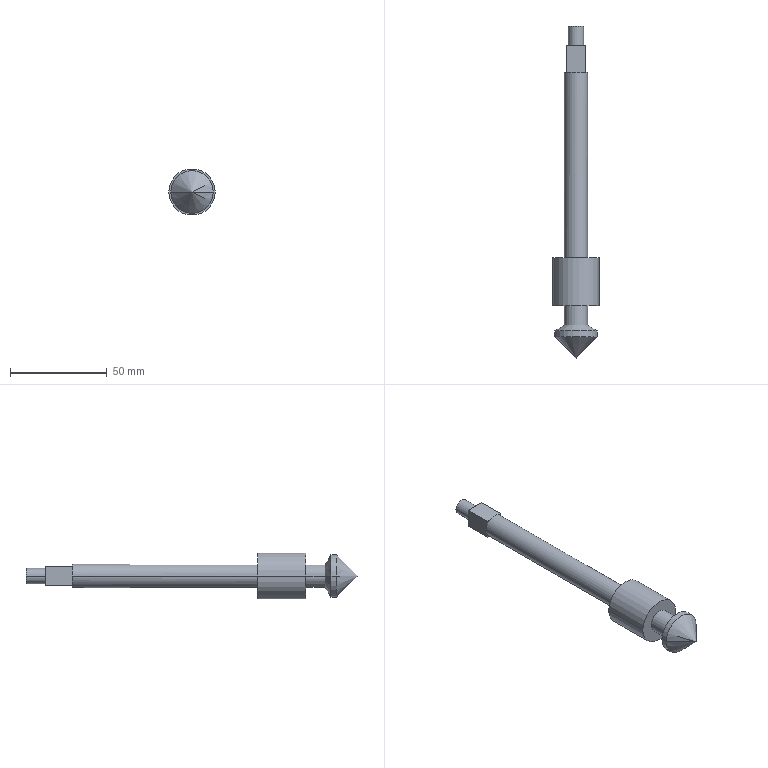Part | SolidWorks | features ICE 2, Revolution 1 | 1 solid | 30 faces | box 24 x 172 x 24 mm | volume 28435 mm3 | plane 16 | cylinder 10 | cone 4 | commonest cylinder face diameters 12 x4 8 x2 22 x2 24 x2
STEP:
#1=CARTESIAN_POINT('',(-4.,172.,0.));
#2=VERTEX_POINT('',#1);
#3=CARTESIAN_POINT('',(4.,172.,0.));
#4=VERTEX_POINT('',#3);
#5=CARTESIAN_POINT('',(0.,172.,0.));
#6=DIRECTION('',(0.,1.,0.));
#7=DIRECTION('',(-1.,0.,0.));
#8=AXIS2_PLACEMENT_3D('',#5,#6,#7);
#9=CIRCLE('',#8,4.);
#10=EDGE_CURVE('',#2,#4,#9,.T.);
#11=ORIENTED_EDGE('',*,*,#10,.F.);
#12=CARTESIAN_POINT('',(-4.,162.,0.));
#13=VERTEX_POINT('',#12);
#14=CARTESIAN_POINT('',(-4.,172.,0.));
#15=DIRECTION('',(0.,-1.,0.));
#16=VECTOR('',#15,1000.);
#17=LINE('',#14,#16);
#18=EDGE_CURVE('',#2,#13,#17,.T.);
#19=ORIENTED_EDGE('',*,*,#18,.T.);
#20=CARTESIAN_POINT('',(4.,162.,0.));
#21=VERTEX_POINT('',#20);
#22=CARTESIAN_POINT('',(0.,162.,0.));
#23=DIRECTION('',(0.,1.,0.));
#24=DIRECTION('',(1.,0.,0.));
#25=AXIS2_PLACEMENT_3D('',#22,#23,#24);
#26=CIRCLE('',#25,4.);
#27=EDGE_CURVE('',#13,#21,#26,.T.);
#28=ORIENTED_EDGE('',*,*,#27,.T.);
#29=CARTESIAN_POINT('',(4.,172.,0.));
#30=DIRECTION('',(0.,-1.,0.));
#31=VECTOR('',#30,1000.);
#32=LINE('',#29,#31);
#33=EDGE_CURVE('',#4,#21,#32,.T.);
#34=ORIENTED_EDGE('',*,*,#33,.F.);
#35=EDGE_LOOP('',(#11,#19,#28,#34));
#36=FACE_OUTER_BOUND('',#35,.T.);
#37=CARTESIAN_POINT('',(0.,172.,0.));
#38=DIRECTION('',(0.,-1.,0.));
#39=DIRECTION('',(1.,0.,0.));
#40=AXIS2_PLACEMENT_3D('',#37,#38,#39);
#41=CYLINDRICAL_SURFACE('',#40,4.);
#42=ADVANCED_FACE('',(#36),#41,.T.);
#43=CARTESIAN_POINT('',(-5.,148.,3.317));
#44=VERTEX_POINT('',#43);
#45=CARTESIAN_POINT('',(-6.,148.,0.));
#46=VERTEX_POINT('',#45);
#47=CARTESIAN_POINT('',(0.,148.,0.));
#48=DIRECTION('',(0.,-1.,0.));
#49=DIRECTION('',(1.,0.,0.));
#50=AXIS2_PLACEMENT_3D('',#47,#48,#49);
#51=CIRCLE('',#50,6.);
#52=EDGE_CURVE('',#44,#46,#51,.T.);
#53=ORIENTED_EDGE('',*,*,#52,.T.);
#54=CARTESIAN_POINT('',(-6.,52.,0.));
#55=VERTEX_POINT('',#54);
#56=CARTESIAN_POINT('',(-6.,-1000.,0.));
#57=DIRECTION('',(0.,-1.,0.));
#58=VECTOR('',#57,1000.);
#59=LINE('',#56,#58);
#60=EDGE_CURVE('',#46,#55,#59,.T.);
#61=ORIENTED_EDGE('',*,*,#60,.T.);
#62=CARTESIAN_POINT('',(6.,52.,0.));
#63=VERTEX_POINT('',#62);
#64=CARTESIAN_POINT('',(0.,52.,0.));
#65=DIRECTION('',(0.,-1.,0.));
#66=DIRECTION('',(1.,0.,0.));
#67=AXIS2_PLACEMENT_3D('',#64,#65,#66);
#68=CIRCLE('',#67,6.);
#69=EDGE_CURVE('',#63,#55,#68,.T.);
#70=ORIENTED_EDGE('',*,*,#69,.F.);
#71=CARTESIAN_POINT('',(6.,148.,0.));
#72=VERTEX_POINT('',#71);
#73=CARTESIAN_POINT('',(6.,-1000.,0.));
#74=DIRECTION('',(0.,-1.,0.));
#75=VECTOR('',#74,1000.);
#76=LINE('',#73,#75);
#77=EDGE_CURVE('',#72,#63,#76,.T.);
#78=ORIENTED_EDGE('',*,*,#77,.F.);
#79=CARTESIAN_POINT('',(5.,148.,3.317));
#80=VERTEX_POINT('',#79);
#81=CARTESIAN_POINT('',(0.,148.,0.));
#82=DIRECTION('',(0.,-1.,0.));
#83=DIRECTION('',(1.,0.,0.));
#84=AXIS2_PLACEMENT_3D('',#81,#82,#83);
#85=CIRCLE('',#84,6.);
#86=EDGE_CURVE('',#72,#80,#85,.T.);
#87=ORIENTED_EDGE('',*,*,#86,.T.);
#88=CARTESIAN_POINT('',(3.317,148.,5.));
#89=VERTEX_POINT('',#88);
#90=CARTESIAN_POINT('',(0.,148.,0.));
#91=DIRECTION('',(0.,-1.,0.));
#92=DIRECTION('',(1.,0.,0.));
#93=AXIS2_PLACEMENT_3D('',#90,#91,#92);
#94=CIRCLE('',#93,6.);
#95=EDGE_CURVE('',#80,#89,#94,.T.);
#96=ORIENTED_EDGE('',*,*,#95,.T.);
#97=CARTESIAN_POINT('',(-3.317,148.,5.));
#98=VERTEX_POINT('',#97);
#99=CARTESIAN_POINT('',(0.,148.,0.));
#100=DIRECTION('',(0.,-1.,0.));
#101=DIRECTION('',(1.,0.,0.));
#102=AXIS2_PLACEMENT_3D('',#99,#100,#101);
#103=CIRCLE('',#102,6.);
#104=EDGE_CURVE('',#89,#98,#103,.T.);
#105=ORIENTED_EDGE('',*,*,#104,.T.);
#106=CARTESIAN_POINT('',(0.,148.,0.));
#107=DIRECTION('',(0.,-1.,0.));
#108=DIRECTION('',(1.,0.,0.));
#109=AXIS2_PLACEMENT_3D('',#106,#107,#108);
#110=CIRCLE('',#109,6.);
#111=EDGE_CURVE('',#98,#44,#110,.T.);
#112=ORIENTED_EDGE('',*,*,#111,.T.);
#113=EDGE_LOOP('',(#53,#61,#70,#78,#87,#96,#105,#112));
#114=FACE_OUTER_BOUND('',#113,.T.);
#115=CARTESIAN_POINT('',(0.,-1000.,0.));
#116=DIRECTION('',(0.,-1.,0.));
#117=DIRECTION('',(1.,0.,0.));
#118=AXIS2_PLACEMENT_3D('',#115,#116,#117);
#119=CYLINDRICAL_SURFACE('',#118,6.);
#120=ADVANCED_FACE('',(#114),#119,.T.);
#121=CARTESIAN_POINT('',(12.,52.,0.));
#122=VERTEX_POINT('',#121);
#123=CARTESIAN_POINT('',(-12.,52.,0.));
#124=VERTEX_POINT('',#123);
#125=CARTESIAN_POINT('',(0.,52.,0.));
#126=DIRECTION('',(0.,-1.,0.));
#127=DIRECTION('',(1.,0.,0.));
#128=AXIS2_PLACEMENT_3D('',#125,#126,#127);
#129=CIRCLE('',#128,12.);
#130=EDGE_CURVE('',#122,#124,#129,.T.);
#131=ORIENTED_EDGE('',*,*,#130,.T.);
#132=CARTESIAN_POINT('',(-12.,27.,0.));
#133=VERTEX_POINT('',#132);
#134=CARTESIAN_POINT('',(-12.,-1000.,0.));
#135=DIRECTION('',(0.,-1.,0.));
#136=VECTOR('',#135,1000.);
#137=LINE('',#134,#136);
#138=EDGE_CURVE('',#124,#133,#137,.T.);
#139=ORIENTED_EDGE('',*,*,#138,.T.);
#140=CARTESIAN_POINT('',(12.,27.,0.));
#141=VERTEX_POINT('',#140);
#142=CARTESIAN_POINT('',(0.,27.,0.));
#143=DIRECTION('',(0.,-1.,0.));
#144=DIRECTION('',(1.,0.,0.));
#145=AXIS2_PLACEMENT_3D('',#142,#143,#144);
#146=CIRCLE('',#145,12.);
#147=EDGE_CURVE('',#141,#133,#146,.T.);
#148=ORIENTED_EDGE('',*,*,#147,.F.);
#149=CARTESIAN_POINT('',(12.,-1000.,0.));
#150=DIRECTION('',(0.,-1.,0.));
#151=VECTOR('',#150,1000.);
#152=LINE('',#149,#151);
#153=EDGE_CURVE('',#122,#141,#152,.T.);
#154=ORIENTED_EDGE('',*,*,#153,.F.);
#155=EDGE_LOOP('',(#131,#139,#148,#154));
#156=FACE_OUTER_BOUND('',#155,.T.);
#157=CARTESIAN_POINT('',(0.,-1000.,0.));
#158=DIRECTION('',(0.,-1.,0.));
#159=DIRECTION('',(1.,0.,0.));
#160=AXIS2_PLACEMENT_3D('',#157,#158,#159);
#161=CYLINDRICAL_SURFACE('',#160,12.);
#162=ADVANCED_FACE('',(#156),#161,.T.);
#163=CARTESIAN_POINT('',(6.,27.,0.));
#164=VERTEX_POINT('',#163);
#165=CARTESIAN_POINT('',(-6.,27.,0.));
#166=VERTEX_POINT('',#165);
#167=CARTESIAN_POINT('',(0.,27.,0.));
#168=DIRECTION('',(0.,-1.,0.));
#169=DIRECTION('',(1.,0.,0.));
#170=AXIS2_PLACEMENT_3D('',#167,#168,#169);
#171=CIRCLE('',#170,6.);
#172=EDGE_CURVE('',#164,#166,#171,.T.);
#173=ORIENTED_EDGE('',*,*,#172,.T.);
#174=CARTESIAN_POINT('',(-6.,17.,0.));
#175=VERTEX_POINT('',#174);
#176=CARTESIAN_POINT('',(-6.,-1000.,0.));
#177=DIRECTION('',(0.,-1.,0.));
#178=VECTOR('',#177,1000.);
#179=LINE('',#176,#178);
#180=EDGE_CURVE('',#166,#175,#179,.T.);
#181=ORIENTED_EDGE('',*,*,#180,.T.);
#182=CARTESIAN_POINT('',(6.,17.,0.));
#183=VERTEX_POINT('',#182);
#184=CARTESIAN_POINT('',(0.,17.,0.));
#185=DIRECTION('',(0.,-1.,0.));
#186=DIRECTION('',(1.,0.,0.));
#187=AXIS2_PLACEMENT_3D('',#184,#185,#186);
#188=CIRCLE('',#187,6.);
#189=EDGE_CURVE('',#183,#175,#188,.T.);
#190=ORIENTED_EDGE('',*,*,#189,.F.);
#191=CARTESIAN_POINT('',(6.,-1000.,0.));
#192=DIRECTION('',(0.,-1.,0.));
#193=VECTOR('',#192,1000.);
#194=LINE('',#191,#193);
#195=EDGE_CURVE('',#164,#183,#194,.T.);
#196=ORIENTED_EDGE('',*,*,#195,.F.);
#197=EDGE_LOOP('',(#173,#181,#190,#196));
#198=FACE_OUTER_BOUND('',#197,.T.);
#199=CARTESIAN_POINT('',(0.,-1000.,0.));
#200=DIRECTION('',(0.,-1.,0.));
#201=DIRECTION('',(1.,0.,0.));
#202=AXIS2_PLACEMENT_3D('',#199,#200,#201);
#203=CYLINDRICAL_SURFACE('',#202,6.);
#204=ADVANCED_FACE('',(#198),#203,.T.);
#205=ORIENTED_EDGE('',*,*,#189,.T.);
#206=CARTESIAN_POINT('',(-11.,14.,0.));
#207=VERTEX_POINT('',#206);
#208=CARTESIAN_POINT('',(-6.,17.,0.));
#209=DIRECTION('',(-0.8575,-0.5145,0.));
#210=VECTOR('',#209,1000.);
#211=LINE('',#208,#210);
#212=EDGE_CURVE('',#175,#207,#211,.T.);
#213=ORIENTED_EDGE('',*,*,#212,.T.);
#214=CARTESIAN_POINT('',(11.,14.,0.));
#215=VERTEX_POINT('',#214);
#216=CARTESIAN_POINT('',(0.,14.,0.));
#217=DIRECTION('',(0.,-1.,0.));
#218=DIRECTION('',(1.,0.,0.));
#219=AXIS2_PLACEMENT_3D('',#216,#217,#218);
#220=CIRCLE('',#219,11.);
#221=EDGE_CURVE('',#215,#207,#220,.T.);
#222=ORIENTED_EDGE('',*,*,#221,.F.);
#223=CARTESIAN_POINT('',(6.,17.,0.));
#224=DIRECTION('',(0.8575,-0.5145,0.));
#225=VECTOR('',#224,1000.);
#226=LINE('',#223,#225);
#227=EDGE_CURVE('',#183,#215,#226,.T.);
#228=ORIENTED_EDGE('',*,*,#227,.F.);
#229=EDGE_LOOP('',(#205,#213,#222,#228));
#230=FACE_OUTER_BOUND('',#229,.T.);
#231=CARTESIAN_POINT('',(0.,17.,0.));
#232=DIRECTION('',(0.,-1.,0.));
#233=DIRECTION('',(1.,0.,0.));
#234=AXIS2_PLACEMENT_3D('',#231,#232,#233);
#235=CONICAL_SURFACE('',#234,6.,1.03);
#236=ADVANCED_FACE('',(#230),#235,.T.);
#237=ORIENTED_EDGE('',*,*,#221,.T.);
#238=CARTESIAN_POINT('',(-11.,11.,0.));
#239=VERTEX_POINT('',#238);
#240=CARTESIAN_POINT('',(-11.,-1000.,0.));
#241=DIRECTION('',(0.,-1.,0.));
#242=VECTOR('',#241,1000.);
#243=LINE('',#240,#242);
#244=EDGE_CURVE('',#207,#239,#243,.T.);
#245=ORIENTED_EDGE('',*,*,#244,.T.);
#246=CARTESIAN_POINT('',(11.,11.,0.));
#247=VERTEX_POINT('',#246);
#248=CARTESIAN_POINT('',(0.,11.,0.));
#249=DIRECTION('',(0.,-1.,0.));
#250=DIRECTION('',(1.,0.,0.));
#251=AXIS2_PLACEMENT_3D('',#248,#249,#250);
#252=CIRCLE('',#251,11.);
#253=EDGE_CURVE('',#247,#239,#252,.T.);
#254=ORIENTED_EDGE('',*,*,#253,.F.);
#255=CARTESIAN_POINT('',(11.,-1000.,0.));
#256=DIRECTION('',(0.,-1.,0.));
#257=VECTOR('',#256,1000.);
#258=LINE('',#255,#257);
#259=EDGE_CURVE('',#215,#247,#258,.T.);
#260=ORIENTED_EDGE('',*,*,#259,.F.);
#261=EDGE_LOOP('',(#237,#245,#254,#260));
#262=FACE_OUTER_BOUND('',#261,.T.);
#263=CARTESIAN_POINT('',(0.,-1000.,0.));
#264=DIRECTION('',(0.,-1.,0.));
#265=DIRECTION('',(1.,0.,0.));
#266=AXIS2_PLACEMENT_3D('',#263,#264,#265);
#267=CYLINDRICAL_SURFACE('',#266,11.);
#268=ADVANCED_FACE('',(#262),#267,.T.);
#269=CARTESIAN_POINT('',(0.,0.,0.));
#270=VERTEX_POINT('',#269);
#271=CARTESIAN_POINT('',(-11.,11.,0.));
#272=DIRECTION('',(-0.7071,0.7071,0.));
#273=VECTOR('',#272,1000.);
#274=LINE('',#271,#273);
#275=EDGE_CURVE('',#270,#239,#274,.T.);
#276=ORIENTED_EDGE('',*,*,#275,.F.);
#277=CARTESIAN_POINT('',(11.,11.,0.));
#278=DIRECTION('',(0.7071,0.7071,0.));
#279=VECTOR('',#278,1000.);
#280=LINE('',#277,#279);
#281=EDGE_CURVE('',#270,#247,#280,.T.);
#282=ORIENTED_EDGE('',*,*,#281,.T.);
#283=ORIENTED_EDGE('',*,*,#253,.T.);
#284=EDGE_LOOP('',(#276,#282,#283));
#285=FACE_OUTER_BOUND('',#284,.T.);
#286=CARTESIAN_POINT('',(0.,11.,0.));
#287=DIRECTION('',(0.,1.,0.));
#288=DIRECTION('',(-1.,0.,0.));
#289=AXIS2_PLACEMENT_3D('',#286,#287,#288);
#290=CONICAL_SURFACE('',#289,11.,0.7854);
#291=ADVANCED_FACE('',(#285),#290,.T.);
#292=CARTESIAN_POINT('',(5.,162.,5.));
#293=VERTEX_POINT('',#292);
#294=CARTESIAN_POINT('',(5.,162.,-5.));
#295=VERTEX_POINT('',#294);
#296=CARTESIAN_POINT('',(5.,162.,5.));
#297=DIRECTION('',(0.,0.,-1.));
#298=VECTOR('',#297,1000.);
#299=LINE('',#296,#298);
#300=EDGE_CURVE('',#293,#295,#299,.T.);
#301=ORIENTED_EDGE('',*,*,#300,.T.);
#302=CARTESIAN_POINT('',(-5.,162.,-5.));
#303=VERTEX_POINT('',#302);
#304=CARTESIAN_POINT('',(-5.,162.,-5.));
#305=DIRECTION('',(-1.,0.,0.));
#306=VECTOR('',#305,1000.);
#307=LINE('',#304,#306);
#308=EDGE_CURVE('',#295,#303,#307,.T.);
#309=ORIENTED_EDGE('',*,*,#308,.T.);
#310=CARTESIAN_POINT('',(-5.,162.,5.));
#311=VERTEX_POINT('',#310);
#312=CARTESIAN_POINT('',(-5.,162.,5.));
#313=DIRECTION('',(0.,0.,1.));
#314=VECTOR('',#313,1000.);
#315=LINE('',#312,#314);
#316=EDGE_CURVE('',#303,#311,#315,.T.);
#317=ORIENTED_EDGE('',*,*,#316,.T.);
#318=CARTESIAN_POINT('',(-5.,162.,5.));
#319=DIRECTION('',(1.,0.,0.));
#320=VECTOR('',#319,1000.);
#321=LINE('',#318,#320);
#322=EDGE_CURVE('',#311,#293,#321,.T.);
#323=ORIENTED_EDGE('',*,*,#322,.T.);
#324=EDGE_LOOP('',(#301,#309,#317,#323));
#325=FACE_OUTER_BOUND('',#324,.T.);
#326=CARTESIAN_POINT('',(0.,162.,0.));
#327=DIRECTION('',(0.,1.,0.));
#328=DIRECTION('',(1.,0.,0.));
#329=AXIS2_PLACEMENT_3D('',#326,#327,#328);
#330=CIRCLE('',#329,4.);
#331=EDGE_CURVE('',#21,#13,#330,.T.);
#332=ORIENTED_EDGE('',*,*,#331,.F.);
#333=ORIENTED_EDGE('',*,*,#27,.F.);
#334=EDGE_LOOP('',(#332,#333));
#335=FACE_BOUND('',#334,.T.);
#336=CARTESIAN_POINT('',(0.,162.,0.));
#337=DIRECTION('',(0.,-1.,0.));
#338=DIRECTION('',(1.,0.,0.));
#339=AXIS2_PLACEMENT_3D('',#336,#337,#338);
#340=PLANE('',#339);
#341=ADVANCED_FACE('',(#325,#335),#340,.F.);
#342=CARTESIAN_POINT('',(5.,148.,-3.317));
#343=VERTEX_POINT('',#342);
#344=CARTESIAN_POINT('',(5.,148.,5.));
#345=DIRECTION('',(0.,0.,-1.));
#346=VECTOR('',#345,1000.);
#347=LINE('',#344,#346);
#348=EDGE_CURVE('',#80,#343,#347,.T.);
#349=ORIENTED_EDGE('',*,*,#348,.F.);
#350=ORIENTED_EDGE('',*,*,#86,.F.);
#351=CARTESIAN_POINT('',(0.,148.,0.));
#352=DIRECTION('',(0.,-1.,0.));
#353=DIRECTION('',(1.,0.,0.));
#354=AXIS2_PLACEMENT_3D('',#351,#352,#353);
#355=CIRCLE('',#354,6.);
#356=EDGE_CURVE('',#343,#72,#355,.T.);
#357=ORIENTED_EDGE('',*,*,#356,.F.);
#358=EDGE_LOOP('',(#349,#350,#357));
#359=FACE_OUTER_BOUND('',#358,.T.);
#360=CARTESIAN_POINT('',(-6.,148.,0.));
#361=DIRECTION('',(0.,-1.,0.));
#362=DIRECTION('',(1.,0.,0.));
#363=AXIS2_PLACEMENT_3D('',#360,#361,#362);
#364=PLANE('',#363);
#365=ADVANCED_FACE('',(#359),#364,.F.);
#366=CARTESIAN_POINT('',(-5.,148.,5.));
#367=DIRECTION('',(1.,0.,0.));
#368=VECTOR('',#367,1000.);
#369=LINE('',#366,#368);
#370=EDGE_CURVE('',#98,#89,#369,.T.);
#371=ORIENTED_EDGE('',*,*,#370,.F.);
#372=ORIENTED_EDGE('',*,*,#104,.F.);
#373=EDGE_LOOP('',(#371,#372));
#374=FACE_OUTER_BOUND('',#373,.T.);
#375=CARTESIAN_POINT('',(-6.,148.,0.));
#376=DIRECTION('',(0.,-1.,0.));
#377=DIRECTION('',(1.,0.,0.));
#378=AXIS2_PLACEMENT_3D('',#375,#376,#377);
#379=PLANE('',#378);
#380=ADVANCED_FACE('',(#374),#379,.F.);
#381=CARTESIAN_POINT('',(-5.,148.,-3.317));
#382=VERTEX_POINT('',#381);
#383=CARTESIAN_POINT('',(-5.,148.,5.));
#384=DIRECTION('',(0.,0.,1.));
#385=VECTOR('',#384,1000.);
#386=LINE('',#383,#385);
#387=EDGE_CURVE('',#382,#44,#386,.T.);
#388=ORIENTED_EDGE('',*,*,#387,.F.);
#389=CARTESIAN_POINT('',(0.,148.,0.));
#390=DIRECTION('',(0.,-1.,0.));
#391=DIRECTION('',(1.,0.,0.));
#392=AXIS2_PLACEMENT_3D('',#389,#390,#391);
#393=CIRCLE('',#392,6.);
#394=EDGE_CURVE('',#46,#382,#393,.T.);
#395=ORIENTED_EDGE('',*,*,#394,.F.);
#396=ORIENTED_EDGE('',*,*,#52,.F.);
#397=EDGE_LOOP('',(#388,#395,#396));
#398=FACE_OUTER_BOUND('',#397,.T.);
#399=CARTESIAN_POINT('',(-6.,148.,0.));
#400=DIRECTION('',(0.,-1.,0.));
#401=DIRECTION('',(1.,0.,0.));
#402=AXIS2_PLACEMENT_3D('',#399,#400,#401);
#403=PLANE('',#402);
#404=ADVANCED_FACE('',(#398),#403,.F.);
#405=CARTESIAN_POINT('',(3.317,148.,-5.));
#406=VERTEX_POINT('',#405);
#407=CARTESIAN_POINT('',(-3.317,148.,-5.));
#408=VERTEX_POINT('',#407);
#409=CARTESIAN_POINT('',(-5.,148.,-5.));
#410=DIRECTION('',(-1.,0.,0.));
#411=VECTOR('',#410,1000.);
#412=LINE('',#409,#411);
#413=EDGE_CURVE('',#406,#408,#412,.T.);
#414=ORIENTED_EDGE('',*,*,#413,.F.);
#415=CARTESIAN_POINT('',(0.,148.,0.));
#416=DIRECTION('',(0.,-1.,0.));
#417=DIRECTION('',(1.,0.,0.));
#418=AXIS2_PLACEMENT_3D('',#415,#416,#417);
#419=CIRCLE('',#418,6.);
#420=EDGE_CURVE('',#408,#406,#419,.T.);
#421=ORIENTED_EDGE('',*,*,#420,.F.);
#422=EDGE_LOOP('',(#414,#421));
#423=FACE_OUTER_BOUND('',#422,.T.);
#424=CARTESIAN_POINT('',(-6.,148.,0.));
#425=DIRECTION('',(0.,-1.,0.));
#426=DIRECTION('',(1.,0.,0.));
#427=AXIS2_PLACEMENT_3D('',#424,#425,#426);
#428=PLANE('',#427);
#429=ADVANCED_FACE('',(#423),#428,.F.);
#430=ORIENTED_EDGE('',*,*,#281,.F.);
#431=ORIENTED_EDGE('',*,*,#275,.T.);
#432=CARTESIAN_POINT('',(0.,11.,0.));
#433=DIRECTION('',(0.,-1.,0.));
#434=DIRECTION('',(1.,0.,0.));
#435=AXIS2_PLACEMENT_3D('',#432,#433,#434);
#436=CIRCLE('',#435,11.);
#437=EDGE_CURVE('',#239,#247,#436,.T.);
#438=ORIENTED_EDGE('',*,*,#437,.T.);
#439=EDGE_LOOP('',(#430,#431,#438));
#440=FACE_OUTER_BOUND('',#439,.T.);
#441=CARTESIAN_POINT('',(0.,11.,0.));
#442=DIRECTION('',(0.,1.,0.));
#443=DIRECTION('',(-1.,0.,0.));
#444=AXIS2_PLACEMENT_3D('',#441,#442,#443);
#445=CONICAL_SURFACE('',#444,11.,0.7854);
#446=ADVANCED_FACE('',(#440),#445,.T.);
#447=ORIENTED_EDGE('',*,*,#244,.F.);
#448=CARTESIAN_POINT('',(0.,14.,0.));
#449=DIRECTION('',(0.,-1.,0.));
#450=DIRECTION('',(1.,0.,0.));
#451=AXIS2_PLACEMENT_3D('',#448,#449,#450);
#452=CIRCLE('',#451,11.);
#453=EDGE_CURVE('',#207,#215,#452,.T.);
#454=ORIENTED_EDGE('',*,*,#453,.T.);
#455=ORIENTED_EDGE('',*,*,#259,.T.);
#456=ORIENTED_EDGE('',*,*,#437,.F.);
#457=EDGE_LOOP('',(#447,#454,#455,#456));
#458=FACE_OUTER_BOUND('',#457,.T.);
#459=CARTESIAN_POINT('',(0.,-1000.,0.));
#460=DIRECTION('',(0.,-1.,0.));
#461=DIRECTION('',(1.,0.,0.));
#462=AXIS2_PLACEMENT_3D('',#459,#460,#461);
#463=CYLINDRICAL_SURFACE('',#462,11.);
#464=ADVANCED_FACE('',(#458),#463,.T.);
#465=ORIENTED_EDGE('',*,*,#212,.F.);
#466=CARTESIAN_POINT('',(0.,17.,0.));
#467=DIRECTION('',(0.,-1.,0.));
#468=DIRECTION('',(1.,0.,0.));
#469=AXIS2_PLACEMENT_3D('',#466,#467,#468);
#470=CIRCLE('',#469,6.);
#471=EDGE_CURVE('',#175,#183,#470,.T.);
#472=ORIENTED_EDGE('',*,*,#471,.T.);
#473=ORIENTED_EDGE('',*,*,#227,.T.);
#474=ORIENTED_EDGE('',*,*,#453,.F.);
#475=EDGE_LOOP('',(#465,#472,#473,#474));
#476=FACE_OUTER_BOUND('',#475,.T.);
#477=CARTESIAN_POINT('',(0.,17.,0.));
#478=DIRECTION('',(0.,-1.,0.));
#479=DIRECTION('',(1.,0.,0.));
#480=AXIS2_PLACEMENT_3D('',#477,#478,#479);
#481=CONICAL_SURFACE('',#480,6.,1.03);
#482=ADVANCED_FACE('',(#476),#481,.T.);
#483=ORIENTED_EDGE('',*,*,#180,.F.);
#484=CARTESIAN_POINT('',(0.,27.,0.));
#485=DIRECTION('',(0.,-1.,0.));
#486=DIRECTION('',(1.,0.,0.));
#487=AXIS2_PLACEMENT_3D('',#484,#485,#486);
#488=CIRCLE('',#487,6.);
#489=EDGE_CURVE('',#166,#164,#488,.T.);
#490=ORIENTED_EDGE('',*,*,#489,.T.);
#491=ORIENTED_EDGE('',*,*,#195,.T.);
#492=ORIENTED_EDGE('',*,*,#471,.F.);
#493=EDGE_LOOP('',(#483,#490,#491,#492));
#494=FACE_OUTER_BOUND('',#493,.T.);
#495=CARTESIAN_POINT('',(0.,-1000.,0.));
#496=DIRECTION('',(0.,-1.,0.));
#497=DIRECTION('',(1.,0.,0.));
#498=AXIS2_PLACEMENT_3D('',#495,#496,#497);
#499=CYLINDRICAL_SURFACE('',#498,6.);
#500=ADVANCED_FACE('',(#494),#499,.T.);
#501=ORIENTED_EDGE('',*,*,#172,.F.);
#502=ORIENTED_EDGE('',*,*,#489,.F.);
#503=EDGE_LOOP('',(#501,#502));
#504=FACE_BOUND('',#503,.T.);
#505=ORIENTED_EDGE('',*,*,#147,.T.);
#506=CARTESIAN_POINT('',(0.,27.,0.));
#507=DIRECTION('',(0.,-1.,0.));
#508=DIRECTION('',(1.,0.,0.));
#509=AXIS2_PLACEMENT_3D('',#506,#507,#508);
#510=CIRCLE('',#509,12.);
#511=EDGE_CURVE('',#133,#141,#510,.T.);
#512=ORIENTED_EDGE('',*,*,#511,.T.);
#513=EDGE_LOOP('',(#505,#512));
#514=FACE_OUTER_BOUND('',#513,.T.);
#515=CARTESIAN_POINT('',(-6.,27.,0.));
#516=DIRECTION('',(0.,1.,0.));
#517=DIRECTION('',(-1.,0.,0.));
#518=AXIS2_PLACEMENT_3D('',#515,#516,#517);
#519=PLANE('',#518);
#520=ADVANCED_FACE('',(#504,#514),#519,.F.);
#521=ORIENTED_EDGE('',*,*,#138,.F.);
#522=CARTESIAN_POINT('',(0.,52.,0.));
#523=DIRECTION('',(0.,-1.,0.));
#524=DIRECTION('',(1.,0.,0.));
#525=AXIS2_PLACEMENT_3D('',#522,#523,#524);
#526=CIRCLE('',#525,12.);
#527=EDGE_CURVE('',#124,#122,#526,.T.);
#528=ORIENTED_EDGE('',*,*,#527,.T.);
#529=ORIENTED_EDGE('',*,*,#153,.T.);
#530=ORIENTED_EDGE('',*,*,#511,.F.);
#531=EDGE_LOOP('',(#521,#528,#529,#530));
#532=FACE_OUTER_BOUND('',#531,.T.);
#533=CARTESIAN_POINT('',(0.,-1000.,0.));
#534=DIRECTION('',(0.,-1.,0.));
#535=DIRECTION('',(1.,0.,0.));
#536=AXIS2_PLACEMENT_3D('',#533,#534,#535);
#537=CYLINDRICAL_SURFACE('',#536,12.);
#538=ADVANCED_FACE('',(#532),#537,.T.);
#539=ORIENTED_EDGE('',*,*,#130,.F.);
#540=ORIENTED_EDGE('',*,*,#527,.F.);
#541=EDGE_LOOP('',(#539,#540));
#542=FACE_OUTER_BOUND('',#541,.T.);
#543=ORIENTED_EDGE('',*,*,#69,.T.);
#544=CARTESIAN_POINT('',(0.,52.,0.));
#545=DIRECTION('',(0.,-1.,0.));
#546=DIRECTION('',(1.,0.,0.));
#547=AXIS2_PLACEMENT_3D('',#544,#545,#546);
#548=CIRCLE('',#547,6.);
#549=EDGE_CURVE('',#55,#63,#548,.T.);
#550=ORIENTED_EDGE('',*,*,#549,.T.);
#551=EDGE_LOOP('',(#543,#550));
#552=FACE_BOUND('',#551,.T.);
#553=CARTESIAN_POINT('',(-12.,52.,0.));
#554=DIRECTION('',(0.,-1.,0.));
#555=DIRECTION('',(1.,0.,0.));
#556=AXIS2_PLACEMENT_3D('',#553,#554,#555);
#557=PLANE('',#556);
#558=ADVANCED_FACE('',(#542,#552),#557,.F.);
#559=ORIENTED_EDGE('',*,*,#60,.F.);
#560=ORIENTED_EDGE('',*,*,#394,.T.);
#561=CARTESIAN_POINT('',(0.,148.,0.));
#562=DIRECTION('',(0.,-1.,0.));
#563=DIRECTION('',(1.,0.,0.));
#564=AXIS2_PLACEMENT_3D('',#561,#562,#563);
#565=CIRCLE('',#564,6.);
#566=EDGE_CURVE('',#382,#408,#565,.T.);
#567=ORIENTED_EDGE('',*,*,#566,.T.);
#568=ORIENTED_EDGE('',*,*,#420,.T.);
#569=CARTESIAN_POINT('',(0.,148.,0.));
#570=DIRECTION('',(0.,-1.,0.));
#571=DIRECTION('',(1.,0.,0.));
#572=AXIS2_PLACEMENT_3D('',#569,#570,#571);
#573=CIRCLE('',#572,6.);
#574=EDGE_CURVE('',#406,#343,#573,.T.);
#575=ORIENTED_EDGE('',*,*,#574,.T.);
#576=ORIENTED_EDGE('',*,*,#356,.T.);
#577=ORIENTED_EDGE('',*,*,#77,.T.);
#578=ORIENTED_EDGE('',*,*,#549,.F.);
#579=EDGE_LOOP('',(#559,#560,#567,#568,#575,#576,#577,#578));
#580=FACE_OUTER_BOUND('',#579,.T.);
#581=CARTESIAN_POINT('',(0.,-1000.,0.));
#582=DIRECTION('',(0.,-1.,0.));
#583=DIRECTION('',(1.,0.,0.));
#584=AXIS2_PLACEMENT_3D('',#581,#582,#583);
#585=CYLINDRICAL_SURFACE('',#584,6.);
#586=ADVANCED_FACE('',(#580),#585,.T.);
#587=ORIENTED_EDGE('',*,*,#95,.F.);
#588=CARTESIAN_POINT('',(5.,148.,5.));
#589=VERTEX_POINT('',#588);
#590=CARTESIAN_POINT('',(5.,148.,5.));
#591=DIRECTION('',(0.,0.,-1.));
#592=VECTOR('',#591,1000.);
#593=LINE('',#590,#592);
#594=EDGE_CURVE('',#589,#80,#593,.T.);
#595=ORIENTED_EDGE('',*,*,#594,.F.);
#596=CARTESIAN_POINT('',(-5.,148.,5.));
#597=DIRECTION('',(1.,0.,0.));
#598=VECTOR('',#597,1000.);
#599=LINE('',#596,#598);
#600=EDGE_CURVE('',#89,#589,#599,.T.);
#601=ORIENTED_EDGE('',*,*,#600,.F.);
#602=EDGE_LOOP('',(#587,#595,#601));
#603=FACE_OUTER_BOUND('',#602,.T.);
#604=CARTESIAN_POINT('',(0.,148.,0.));
#605=DIRECTION('',(0.,-1.,0.));
#606=DIRECTION('',(1.,0.,0.));
#607=AXIS2_PLACEMENT_3D('',#604,#605,#606);
#608=PLANE('',#607);
#609=ADVANCED_FACE('',(#603),#608,.T.);
#610=ORIENTED_EDGE('',*,*,#111,.F.);
#611=CARTESIAN_POINT('',(-5.,148.,5.));
#612=VERTEX_POINT('',#611);
#613=CARTESIAN_POINT('',(-5.,148.,5.));
#614=DIRECTION('',(1.,0.,0.));
#615=VECTOR('',#614,1000.);
#616=LINE('',#613,#615);
#617=EDGE_CURVE('',#612,#98,#616,.T.);
#618=ORIENTED_EDGE('',*,*,#617,.F.);
#619=CARTESIAN_POINT('',(-5.,148.,5.));
#620=DIRECTION('',(0.,0.,1.));
#621=VECTOR('',#620,1000.);
#622=LINE('',#619,#621);
#623=EDGE_CURVE('',#44,#612,#622,.T.);
#624=ORIENTED_EDGE('',*,*,#623,.F.);
#625=EDGE_LOOP('',(#610,#618,#624));
#626=FACE_OUTER_BOUND('',#625,.T.);
#627=CARTESIAN_POINT('',(0.,148.,0.));
#628=DIRECTION('',(0.,-1.,0.));
#629=DIRECTION('',(1.,0.,0.));
#630=AXIS2_PLACEMENT_3D('',#627,#628,#629);
#631=PLANE('',#630);
#632=ADVANCED_FACE('',(#626),#631,.T.);
#633=ORIENTED_EDGE('',*,*,#566,.F.);
#634=CARTESIAN_POINT('',(-5.,148.,-5.));
#635=VERTEX_POINT('',#634);
#636=CARTESIAN_POINT('',(-5.,148.,5.));
#637=DIRECTION('',(0.,0.,1.));
#638=VECTOR('',#637,1000.);
#639=LINE('',#636,#638);
#640=EDGE_CURVE('',#635,#382,#639,.T.);
#641=ORIENTED_EDGE('',*,*,#640,.F.);
#642=CARTESIAN_POINT('',(-5.,148.,-5.));
#643=DIRECTION('',(-1.,0.,0.));
#644=VECTOR('',#643,1000.);
#645=LINE('',#642,#644);
#646=EDGE_CURVE('',#408,#635,#645,.T.);
#647=ORIENTED_EDGE('',*,*,#646,.F.);
#648=EDGE_LOOP('',(#633,#641,#647));
#649=FACE_OUTER_BOUND('',#648,.T.);
#650=CARTESIAN_POINT('',(0.,148.,0.));
#651=DIRECTION('',(0.,-1.,0.));
#652=DIRECTION('',(1.,0.,0.));
#653=AXIS2_PLACEMENT_3D('',#650,#651,#652);
#654=PLANE('',#653);
#655=ADVANCED_FACE('',(#649),#654,.T.);
#656=ORIENTED_EDGE('',*,*,#574,.F.);
#657=CARTESIAN_POINT('',(5.,148.,-5.));
#658=VERTEX_POINT('',#657);
#659=CARTESIAN_POINT('',(-5.,148.,-5.));
#660=DIRECTION('',(-1.,0.,0.));
#661=VECTOR('',#660,1000.);
#662=LINE('',#659,#661);
#663=EDGE_CURVE('',#658,#406,#662,.T.);
#664=ORIENTED_EDGE('',*,*,#663,.F.);
#665=CARTESIAN_POINT('',(5.,148.,5.));
#666=DIRECTION('',(0.,0.,-1.));
#667=VECTOR('',#666,1000.);
#668=LINE('',#665,#667);
#669=EDGE_CURVE('',#343,#658,#668,.T.);
#670=ORIENTED_EDGE('',*,*,#669,.F.);
#671=EDGE_LOOP('',(#656,#664,#670));
#672=FACE_OUTER_BOUND('',#671,.T.);
#673=CARTESIAN_POINT('',(0.,148.,0.));
#674=DIRECTION('',(0.,-1.,0.));
#675=DIRECTION('',(1.,0.,0.));
#676=AXIS2_PLACEMENT_3D('',#673,#674,#675);
#677=PLANE('',#676);
#678=ADVANCED_FACE('',(#672),#677,.T.);
#679=ORIENTED_EDGE('',*,*,#594,.T.);
#680=ORIENTED_EDGE('',*,*,#348,.T.);
#681=ORIENTED_EDGE('',*,*,#669,.T.);
#682=CARTESIAN_POINT('',(5.,162.,-5.));
#683=DIRECTION('',(0.,-1.,0.));
#684=VECTOR('',#683,1000.);
#685=LINE('',#682,#684);
#686=EDGE_CURVE('',#295,#658,#685,.T.);
#687=ORIENTED_EDGE('',*,*,#686,.F.);
#688=ORIENTED_EDGE('',*,*,#300,.F.);
#689=CARTESIAN_POINT('',(5.,162.,5.));
#690=DIRECTION('',(0.,-1.,0.));
#691=VECTOR('',#690,1000.);
#692=LINE('',#689,#691);
#693=EDGE_CURVE('',#293,#589,#692,.T.);
#694=ORIENTED_EDGE('',*,*,#693,.T.);
#695=EDGE_LOOP('',(#679,#680,#681,#687,#688,#694));
#696=FACE_OUTER_BOUND('',#695,.T.);
#697=CARTESIAN_POINT('',(5.,162.,5.));
#698=DIRECTION('',(-1.,0.,0.));
#699=DIRECTION('',(0.,-1.,0.));
#700=AXIS2_PLACEMENT_3D('',#697,#698,#699);
#701=PLANE('',#700);
#702=ADVANCED_FACE('',(#696),#701,.F.);
#703=ORIENTED_EDGE('',*,*,#663,.T.);
#704=ORIENTED_EDGE('',*,*,#413,.T.);
#705=ORIENTED_EDGE('',*,*,#646,.T.);
#706=CARTESIAN_POINT('',(-5.,162.,-5.));
#707=DIRECTION('',(0.,-1.,0.));
#708=VECTOR('',#707,1000.);
#709=LINE('',#706,#708);
#710=EDGE_CURVE('',#303,#635,#709,.T.);
#711=ORIENTED_EDGE('',*,*,#710,.F.);
#712=ORIENTED_EDGE('',*,*,#308,.F.);
#713=ORIENTED_EDGE('',*,*,#686,.T.);
#714=EDGE_LOOP('',(#703,#704,#705,#711,#712,#713));
#715=FACE_OUTER_BOUND('',#714,.T.);
#716=CARTESIAN_POINT('',(-5.,162.,-5.));
#717=DIRECTION('',(0.,0.,1.));
#718=DIRECTION('',(1.,0.,0.));
#719=AXIS2_PLACEMENT_3D('',#716,#717,#718);
#720=PLANE('',#719);
#721=ADVANCED_FACE('',(#715),#720,.F.);
#722=ORIENTED_EDGE('',*,*,#640,.T.);
#723=ORIENTED_EDGE('',*,*,#387,.T.);
#724=ORIENTED_EDGE('',*,*,#623,.T.);
#725=CARTESIAN_POINT('',(-5.,162.,5.));
#726=DIRECTION('',(0.,-1.,0.));
#727=VECTOR('',#726,1000.);
#728=LINE('',#725,#727);
#729=EDGE_CURVE('',#311,#612,#728,.T.);
#730=ORIENTED_EDGE('',*,*,#729,.F.);
#731=ORIENTED_EDGE('',*,*,#316,.F.);
#732=ORIENTED_EDGE('',*,*,#710,.T.);
#733=EDGE_LOOP('',(#722,#723,#724,#730,#731,#732));
#734=FACE_OUTER_BOUND('',#733,.T.);
#735=CARTESIAN_POINT('',(-5.,162.,5.));
#736=DIRECTION('',(1.,0.,0.));
#737=DIRECTION('',(0.,1.,0.));
#738=AXIS2_PLACEMENT_3D('',#735,#736,#737);
#739=PLANE('',#738);
#740=ADVANCED_FACE('',(#734),#739,.F.);
#741=ORIENTED_EDGE('',*,*,#617,.T.);
#742=ORIENTED_EDGE('',*,*,#370,.T.);
#743=ORIENTED_EDGE('',*,*,#600,.T.);
#744=ORIENTED_EDGE('',*,*,#693,.F.);
#745=ORIENTED_EDGE('',*,*,#322,.F.);
#746=ORIENTED_EDGE('',*,*,#729,.T.);
#747=EDGE_LOOP('',(#741,#742,#743,#744,#745,#746));
#748=FACE_OUTER_BOUND('',#747,.T.);
#749=CARTESIAN_POINT('',(-5.,162.,5.));
#750=DIRECTION('',(0.,0.,-1.));
#751=DIRECTION('',(-1.,0.,0.));
#752=AXIS2_PLACEMENT_3D('',#749,#750,#751);
#753=PLANE('',#752);
#754=ADVANCED_FACE('',(#748),#753,.F.);
#755=ORIENTED_EDGE('',*,*,#18,.F.);
#756=CARTESIAN_POINT('',(0.,172.,0.));
#757=DIRECTION('',(0.,1.,0.));
#758=DIRECTION('',(-1.,0.,0.));
#759=AXIS2_PLACEMENT_3D('',#756,#757,#758);
#760=CIRCLE('',#759,4.);
#761=EDGE_CURVE('',#4,#2,#760,.T.);
#762=ORIENTED_EDGE('',*,*,#761,.F.);
#763=ORIENTED_EDGE('',*,*,#33,.T.);
#764=ORIENTED_EDGE('',*,*,#331,.T.);
#765=EDGE_LOOP('',(#755,#762,#763,#764));
#766=FACE_OUTER_BOUND('',#765,.T.);
#767=CARTESIAN_POINT('',(0.,172.,0.));
#768=DIRECTION('',(0.,-1.,0.));
#769=DIRECTION('',(1.,0.,0.));
#770=AXIS2_PLACEMENT_3D('',#767,#768,#769);
#771=CYLINDRICAL_SURFACE('',#770,4.);
#772=ADVANCED_FACE('',(#766),#771,.T.);
#773=ORIENTED_EDGE('',*,*,#761,.T.);
#774=ORIENTED_EDGE('',*,*,#10,.T.);
#775=EDGE_LOOP('',(#773,#774));
#776=FACE_OUTER_BOUND('',#775,.T.);
#777=CARTESIAN_POINT('',(0.,172.,0.));
#778=DIRECTION('',(0.,1.,0.));
#779=DIRECTION('',(-1.,0.,0.));
#780=AXIS2_PLACEMENT_3D('',#777,#778,#779);
#781=PLANE('',#780);
#782=ADVANCED_FACE('',(#776),#781,.T.);
#783=CLOSED_SHELL('',(#42,#120,#162,#204,#236,#268,#291,#341,#365,#380,#404,#429,#446,#464,#482,#500,#520,#538,#558,#586,#609,#632,#655,#678,#702,#721,#740,#754,#772,#782));
#784=MANIFOLD_SOLID_BREP('',#783);
#785=CARTESIAN_POINT('',(0.,0.,0.));
#786=DIRECTION('',(0.,0.,1.));
#787=DIRECTION('',(1.,0.,0.));
#788=AXIS2_PLACEMENT_3D('',#785,#786,#787);
#789=(LENGTH_UNIT()NAMED_UNIT(*)SI_UNIT(.MILLI.,.METRE.));
#790=UNCERTAINTY_MEASURE_WITH_UNIT(LENGTH_MEASURE(0.00001),#789,'','');
#791=(NAMED_UNIT(*)PLANE_ANGLE_UNIT()SI_UNIT($,.RADIAN.));
#792=(NAMED_UNIT(*)SI_UNIT($,.STERADIAN.)SOLID_ANGLE_UNIT());
#793=(GEOMETRIC_REPRESENTATION_CONTEXT(3)GLOBAL_UNCERTAINTY_ASSIGNED_CONTEXT((#790))GLOBAL_UNIT_ASSIGNED_CONTEXT((#789,#791,#792))REPRESENTATION_CONTEXT('',''));
#794=ADVANCED_BREP_SHAPE_REPRESENTATION('',(#784,#788),#793);